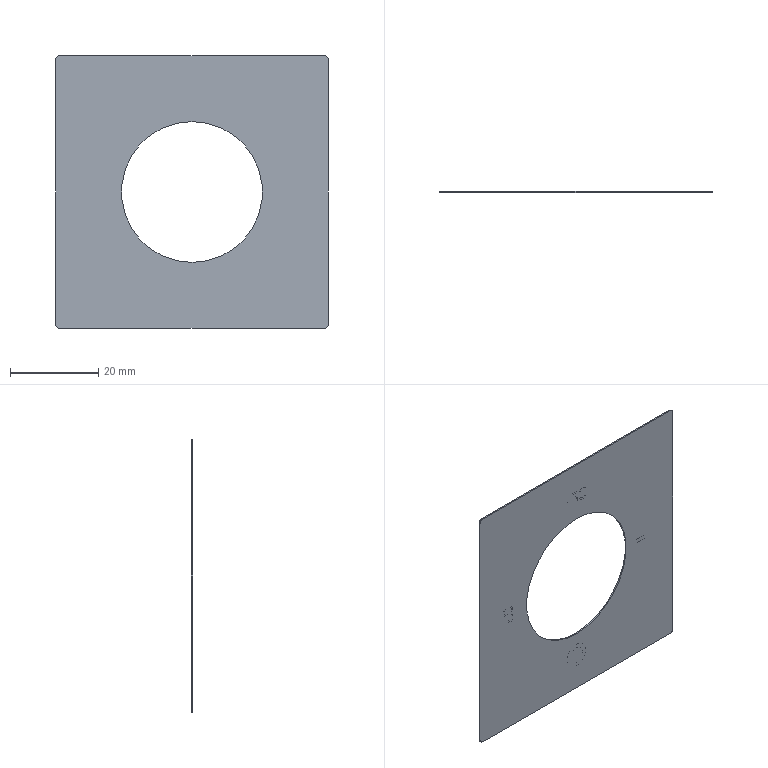Part | STEP file | PCS-01CC-2_1_2.stp | 1 solid | 82 faces | box 62 x 0.3 x 62 mm | volume 908.364 mm3 | plane 50 | spline 22 | cylinder 10 | commonest cylinder face diameters 2 x4 4 x2 6 x2 32 x2